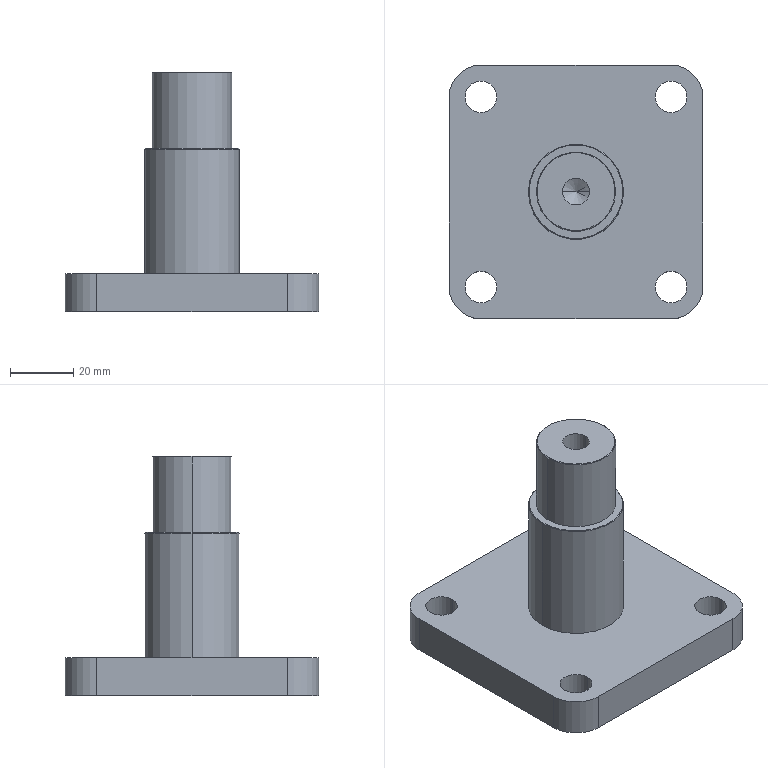Part | NX | features BREP 2 | 2 solids | 38 faces | box 80 x 80 x 75.5 mm | volume 109108 mm3 | cylinder 22 | plane 10 | cone 6 | commonest cylinder face diameters 10 x8 25 x6 20 x4 8.5 x2 30 x2
STEP:
#1=CARTESIAN_POINT('',(-25.,30.,0.));
#2=VERTEX_POINT('',#1);
#3=CARTESIAN_POINT('',(-35.,30.,0.));
#4=VERTEX_POINT('',#3);
#5=CARTESIAN_POINT('',(-30.,30.,0.));
#6=DIRECTION('',(0.,0.,-1.));
#7=DIRECTION('',(-1.,0.,0.));
#8=AXIS2_PLACEMENT_3D('',#5,#6,#7);
#9=CIRCLE('',#8,5.);
#10=EDGE_CURVE('',#2,#4,#9,.T.);
#11=ORIENTED_EDGE('',*,*,#10,.T.);
#12=CARTESIAN_POINT('',(-35.,30.,12.));
#13=VERTEX_POINT('',#12);
#14=CARTESIAN_POINT('',(-35.,30.,12.));
#15=DIRECTION('',(0.,0.,1.));
#16=VECTOR('',#15,1000.);
#17=LINE('',#14,#16);
#18=EDGE_CURVE('',#13,#4,#17,.F.);
#19=ORIENTED_EDGE('',*,*,#18,.F.);
#20=CARTESIAN_POINT('',(-25.,30.,12.));
#21=VERTEX_POINT('',#20);
#22=CARTESIAN_POINT('',(-30.,30.,12.));
#23=DIRECTION('',(0.,0.,1.));
#24=DIRECTION('',(1.,0.,0.));
#25=AXIS2_PLACEMENT_3D('',#22,#23,#24);
#26=CIRCLE('',#25,5.);
#27=EDGE_CURVE('',#13,#21,#26,.T.);
#28=ORIENTED_EDGE('',*,*,#27,.T.);
#29=CARTESIAN_POINT('',(-25.,30.,12.));
#30=DIRECTION('',(0.,0.,1.));
#31=VECTOR('',#30,1000.);
#32=LINE('',#29,#31);
#33=EDGE_CURVE('',#21,#2,#32,.F.);
#34=ORIENTED_EDGE('',*,*,#33,.T.);
#35=EDGE_LOOP('',(#11,#19,#28,#34));
#36=FACE_BOUND('',#35,.T.);
#37=CARTESIAN_POINT('',(-30.,30.,12.));
#38=DIRECTION('',(0.,0.,1.));
#39=DIRECTION('',(1.,0.,0.));
#40=AXIS2_PLACEMENT_3D('',#37,#38,#39);
#41=CYLINDRICAL_SURFACE('',#40,5.);
#42=ADVANCED_FACE('',(#36),#41,.F.);
#43=CARTESIAN_POINT('',(35.,-30.,0.));
#44=VERTEX_POINT('',#43);
#45=CARTESIAN_POINT('',(25.,-30.,0.));
#46=VERTEX_POINT('',#45);
#47=CARTESIAN_POINT('',(30.,-30.,0.));
#48=DIRECTION('',(0.,0.,-1.));
#49=DIRECTION('',(-1.,0.,0.));
#50=AXIS2_PLACEMENT_3D('',#47,#48,#49);
#51=CIRCLE('',#50,5.);
#52=EDGE_CURVE('',#44,#46,#51,.T.);
#53=ORIENTED_EDGE('',*,*,#52,.T.);
#54=CARTESIAN_POINT('',(25.,-30.,12.));
#55=VERTEX_POINT('',#54);
#56=CARTESIAN_POINT('',(25.,-30.,12.));
#57=DIRECTION('',(0.,0.,1.));
#58=VECTOR('',#57,1000.);
#59=LINE('',#56,#58);
#60=EDGE_CURVE('',#55,#46,#59,.F.);
#61=ORIENTED_EDGE('',*,*,#60,.F.);
#62=CARTESIAN_POINT('',(35.,-30.,12.));
#63=VERTEX_POINT('',#62);
#64=CARTESIAN_POINT('',(30.,-30.,12.));
#65=DIRECTION('',(0.,0.,1.));
#66=DIRECTION('',(1.,0.,0.));
#67=AXIS2_PLACEMENT_3D('',#64,#65,#66);
#68=CIRCLE('',#67,5.);
#69=EDGE_CURVE('',#55,#63,#68,.T.);
#70=ORIENTED_EDGE('',*,*,#69,.T.);
#71=CARTESIAN_POINT('',(35.,-30.,12.));
#72=DIRECTION('',(0.,0.,1.));
#73=VECTOR('',#72,1000.);
#74=LINE('',#71,#73);
#75=EDGE_CURVE('',#63,#44,#74,.F.);
#76=ORIENTED_EDGE('',*,*,#75,.T.);
#77=EDGE_LOOP('',(#53,#61,#70,#76));
#78=FACE_BOUND('',#77,.T.);
#79=CARTESIAN_POINT('',(30.,-30.,12.));
#80=DIRECTION('',(0.,0.,1.));
#81=DIRECTION('',(1.,0.,0.));
#82=AXIS2_PLACEMENT_3D('',#79,#80,#81);
#83=CYLINDRICAL_SURFACE('',#82,5.);
#84=ADVANCED_FACE('',(#78),#83,.F.);
#85=CARTESIAN_POINT('',(-25.,-30.,0.));
#86=VERTEX_POINT('',#85);
#87=CARTESIAN_POINT('',(-35.,-30.,0.));
#88=VERTEX_POINT('',#87);
#89=CARTESIAN_POINT('',(-30.,-30.,0.));
#90=DIRECTION('',(0.,0.,-1.));
#91=DIRECTION('',(-1.,0.,0.));
#92=AXIS2_PLACEMENT_3D('',#89,#90,#91);
#93=CIRCLE('',#92,5.);
#94=EDGE_CURVE('',#86,#88,#93,.T.);
#95=ORIENTED_EDGE('',*,*,#94,.T.);
#96=CARTESIAN_POINT('',(-35.,-30.,12.));
#97=VERTEX_POINT('',#96);
#98=CARTESIAN_POINT('',(-35.,-30.,12.));
#99=DIRECTION('',(0.,0.,1.));
#100=VECTOR('',#99,1000.);
#101=LINE('',#98,#100);
#102=EDGE_CURVE('',#97,#88,#101,.F.);
#103=ORIENTED_EDGE('',*,*,#102,.F.);
#104=CARTESIAN_POINT('',(-25.,-30.,12.));
#105=VERTEX_POINT('',#104);
#106=CARTESIAN_POINT('',(-30.,-30.,12.));
#107=DIRECTION('',(0.,0.,1.));
#108=DIRECTION('',(1.,0.,0.));
#109=AXIS2_PLACEMENT_3D('',#106,#107,#108);
#110=CIRCLE('',#109,5.);
#111=EDGE_CURVE('',#97,#105,#110,.T.);
#112=ORIENTED_EDGE('',*,*,#111,.T.);
#113=CARTESIAN_POINT('',(-25.,-30.,12.));
#114=DIRECTION('',(0.,0.,1.));
#115=VECTOR('',#114,1000.);
#116=LINE('',#113,#115);
#117=EDGE_CURVE('',#105,#86,#116,.F.);
#118=ORIENTED_EDGE('',*,*,#117,.T.);
#119=EDGE_LOOP('',(#95,#103,#112,#118));
#120=FACE_BOUND('',#119,.T.);
#121=CARTESIAN_POINT('',(-30.,-30.,12.));
#122=DIRECTION('',(0.,0.,1.));
#123=DIRECTION('',(1.,0.,0.));
#124=AXIS2_PLACEMENT_3D('',#121,#122,#123);
#125=CYLINDRICAL_SURFACE('',#124,5.);
#126=ADVANCED_FACE('',(#120),#125,.F.);
#127=CARTESIAN_POINT('',(35.,30.,0.));
#128=VERTEX_POINT('',#127);
#129=CARTESIAN_POINT('',(25.,30.,0.));
#130=VERTEX_POINT('',#129);
#131=CARTESIAN_POINT('',(30.,30.,0.));
#132=DIRECTION('',(0.,0.,-1.));
#133=DIRECTION('',(-1.,0.,0.));
#134=AXIS2_PLACEMENT_3D('',#131,#132,#133);
#135=CIRCLE('',#134,5.);
#136=EDGE_CURVE('',#128,#130,#135,.T.);
#137=ORIENTED_EDGE('',*,*,#136,.T.);
#138=CARTESIAN_POINT('',(25.,30.,12.));
#139=VERTEX_POINT('',#138);
#140=CARTESIAN_POINT('',(25.,30.,12.));
#141=DIRECTION('',(0.,0.,1.));
#142=VECTOR('',#141,1000.);
#143=LINE('',#140,#142);
#144=EDGE_CURVE('',#139,#130,#143,.F.);
#145=ORIENTED_EDGE('',*,*,#144,.F.);
#146=CARTESIAN_POINT('',(35.,30.,12.));
#147=VERTEX_POINT('',#146);
#148=CARTESIAN_POINT('',(30.,30.,12.));
#149=DIRECTION('',(0.,0.,1.));
#150=DIRECTION('',(1.,0.,0.));
#151=AXIS2_PLACEMENT_3D('',#148,#149,#150);
#152=CIRCLE('',#151,5.);
#153=EDGE_CURVE('',#139,#147,#152,.T.);
#154=ORIENTED_EDGE('',*,*,#153,.T.);
#155=CARTESIAN_POINT('',(35.,30.,12.));
#156=DIRECTION('',(0.,0.,1.));
#157=VECTOR('',#156,1000.);
#158=LINE('',#155,#157);
#159=EDGE_CURVE('',#147,#128,#158,.F.);
#160=ORIENTED_EDGE('',*,*,#159,.T.);
#161=EDGE_LOOP('',(#137,#145,#154,#160));
#162=FACE_BOUND('',#161,.T.);
#163=CARTESIAN_POINT('',(30.,30.,12.));
#164=DIRECTION('',(0.,0.,1.));
#165=DIRECTION('',(1.,0.,0.));
#166=AXIS2_PLACEMENT_3D('',#163,#164,#165);
#167=CYLINDRICAL_SURFACE('',#166,5.);
#168=ADVANCED_FACE('',(#162),#167,.F.);
#169=CARTESIAN_POINT('',(-12.5,0.,0.));
#170=VERTEX_POINT('',#169);
#171=CARTESIAN_POINT('',(12.5,0.,0.));
#172=VERTEX_POINT('',#171);
#173=CARTESIAN_POINT('',(0.,0.,0.));
#174=DIRECTION('',(0.,0.,1.));
#175=DIRECTION('',(1.,0.,0.));
#176=AXIS2_PLACEMENT_3D('',#173,#174,#175);
#177=CIRCLE('',#176,12.5);
#178=EDGE_CURVE('',#170,#172,#177,.T.);
#179=ORIENTED_EDGE('',*,*,#178,.F.);
#180=CARTESIAN_POINT('',(-12.5,0.,12.));
#181=VERTEX_POINT('',#180);
#182=CARTESIAN_POINT('',(-12.5,0.,0.));
#183=DIRECTION('',(0.,0.,1.));
#184=VECTOR('',#183,1000.);
#185=LINE('',#182,#184);
#186=EDGE_CURVE('',#181,#170,#185,.F.);
#187=ORIENTED_EDGE('',*,*,#186,.F.);
#188=CARTESIAN_POINT('',(12.5,0.,12.));
#189=VERTEX_POINT('',#188);
#190=CARTESIAN_POINT('',(0.,0.,12.));
#191=DIRECTION('',(0.,0.,1.));
#192=DIRECTION('',(1.,0.,0.));
#193=AXIS2_PLACEMENT_3D('',#190,#191,#192);
#194=CIRCLE('',#193,12.5);
#195=EDGE_CURVE('',#181,#189,#194,.T.);
#196=ORIENTED_EDGE('',*,*,#195,.T.);
#197=CARTESIAN_POINT('',(12.5,0.,0.));
#198=DIRECTION('',(0.,0.,1.));
#199=VECTOR('',#198,1000.);
#200=LINE('',#197,#199);
#201=EDGE_CURVE('',#189,#172,#200,.F.);
#202=ORIENTED_EDGE('',*,*,#201,.T.);
#203=EDGE_LOOP('',(#179,#187,#196,#202));
#204=FACE_BOUND('',#203,.T.);
#205=CARTESIAN_POINT('',(0.,0.,0.));
#206=DIRECTION('',(0.,0.,1.));
#207=DIRECTION('',(1.,0.,0.));
#208=AXIS2_PLACEMENT_3D('',#205,#206,#207);
#209=CYLINDRICAL_SURFACE('',#208,12.5);
#210=ADVANCED_FACE('',(#204),#209,.F.);
#211=CARTESIAN_POINT('',(-30.,-40.,12.));
#212=VERTEX_POINT('',#211);
#213=CARTESIAN_POINT('',(30.,-40.,12.));
#214=VERTEX_POINT('',#213);
#215=CARTESIAN_POINT('',(-40.,-40.,12.));
#216=DIRECTION('',(1.,0.,0.));
#217=VECTOR('',#216,1000.);
#218=LINE('',#215,#217);
#219=EDGE_CURVE('',#212,#214,#218,.T.);
#220=ORIENTED_EDGE('',*,*,#219,.T.);
#221=CARTESIAN_POINT('',(40.,-30.,12.));
#222=VERTEX_POINT('',#221);
#223=CARTESIAN_POINT('',(30.,-30.,12.));
#224=DIRECTION('',(0.,0.,1.));
#225=DIRECTION('',(-1.,0.,0.));
#226=AXIS2_PLACEMENT_3D('',#223,#224,#225);
#227=CIRCLE('',#226,10.);
#228=EDGE_CURVE('',#214,#222,#227,.T.);
#229=ORIENTED_EDGE('',*,*,#228,.T.);
#230=CARTESIAN_POINT('',(40.,30.,12.));
#231=VERTEX_POINT('',#230);
#232=CARTESIAN_POINT('',(40.,-40.,12.));
#233=DIRECTION('',(0.,1.,0.));
#234=VECTOR('',#233,1000.);
#235=LINE('',#232,#234);
#236=EDGE_CURVE('',#222,#231,#235,.T.);
#237=ORIENTED_EDGE('',*,*,#236,.T.);
#238=CARTESIAN_POINT('',(30.,40.,12.));
#239=VERTEX_POINT('',#238);
#240=CARTESIAN_POINT('',(30.,30.,12.));
#241=DIRECTION('',(0.,0.,1.));
#242=DIRECTION('',(-1.,0.,0.));
#243=AXIS2_PLACEMENT_3D('',#240,#241,#242);
#244=CIRCLE('',#243,10.);
#245=EDGE_CURVE('',#231,#239,#244,.T.);
#246=ORIENTED_EDGE('',*,*,#245,.T.);
#247=CARTESIAN_POINT('',(-30.,40.,12.));
#248=VERTEX_POINT('',#247);
#249=CARTESIAN_POINT('',(-40.,40.,12.));
#250=DIRECTION('',(-1.,0.,0.));
#251=VECTOR('',#250,1000.);
#252=LINE('',#249,#251);
#253=EDGE_CURVE('',#239,#248,#252,.T.);
#254=ORIENTED_EDGE('',*,*,#253,.T.);
#255=CARTESIAN_POINT('',(-40.,30.,12.));
#256=VERTEX_POINT('',#255);
#257=CARTESIAN_POINT('',(-30.,30.,12.));
#258=DIRECTION('',(0.,0.,1.));
#259=DIRECTION('',(-1.,0.,0.));
#260=AXIS2_PLACEMENT_3D('',#257,#258,#259);
#261=CIRCLE('',#260,10.);
#262=EDGE_CURVE('',#248,#256,#261,.T.);
#263=ORIENTED_EDGE('',*,*,#262,.T.);
#264=CARTESIAN_POINT('',(-40.,-30.,12.));
#265=VERTEX_POINT('',#264);
#266=CARTESIAN_POINT('',(-40.,-40.,12.));
#267=DIRECTION('',(0.,-1.,0.));
#268=VECTOR('',#267,1000.);
#269=LINE('',#266,#268);
#270=EDGE_CURVE('',#256,#265,#269,.T.);
#271=ORIENTED_EDGE('',*,*,#270,.T.);
#272=CARTESIAN_POINT('',(-30.,-30.,12.));
#273=DIRECTION('',(0.,0.,1.));
#274=DIRECTION('',(-1.,0.,0.));
#275=AXIS2_PLACEMENT_3D('',#272,#273,#274);
#276=CIRCLE('',#275,10.);
#277=EDGE_CURVE('',#265,#212,#276,.T.);
#278=ORIENTED_EDGE('',*,*,#277,.T.);
#279=EDGE_LOOP('',(#220,#229,#237,#246,#254,#263,#271,#278));
#280=FACE_BOUND('',#279,.T.);
#281=CARTESIAN_POINT('',(-30.,-30.,12.));
#282=DIRECTION('',(0.,0.,1.));
#283=DIRECTION('',(1.,0.,0.));
#284=AXIS2_PLACEMENT_3D('',#281,#282,#283);
#285=CIRCLE('',#284,5.);
#286=EDGE_CURVE('',#105,#97,#285,.T.);
#287=ORIENTED_EDGE('',*,*,#286,.F.);
#288=ORIENTED_EDGE('',*,*,#111,.F.);
#289=EDGE_LOOP('',(#287,#288));
#290=FACE_BOUND('',#289,.T.);
#291=CARTESIAN_POINT('',(30.,30.,12.));
#292=DIRECTION('',(0.,0.,1.));
#293=DIRECTION('',(1.,0.,0.));
#294=AXIS2_PLACEMENT_3D('',#291,#292,#293);
#295=CIRCLE('',#294,5.);
#296=EDGE_CURVE('',#147,#139,#295,.T.);
#297=ORIENTED_EDGE('',*,*,#296,.F.);
#298=ORIENTED_EDGE('',*,*,#153,.F.);
#299=EDGE_LOOP('',(#297,#298));
#300=FACE_BOUND('',#299,.T.);
#301=CARTESIAN_POINT('',(0.,0.,12.));
#302=DIRECTION('',(0.,0.,1.));
#303=DIRECTION('',(1.,0.,0.));
#304=AXIS2_PLACEMENT_3D('',#301,#302,#303);
#305=CIRCLE('',#304,12.5);
#306=EDGE_CURVE('',#189,#181,#305,.T.);
#307=ORIENTED_EDGE('',*,*,#306,.F.);
#308=ORIENTED_EDGE('',*,*,#195,.F.);
#309=EDGE_LOOP('',(#307,#308));
#310=FACE_BOUND('',#309,.T.);
#311=CARTESIAN_POINT('',(30.,-30.,12.));
#312=DIRECTION('',(0.,0.,1.));
#313=DIRECTION('',(1.,0.,0.));
#314=AXIS2_PLACEMENT_3D('',#311,#312,#313);
#315=CIRCLE('',#314,5.);
#316=EDGE_CURVE('',#63,#55,#315,.T.);
#317=ORIENTED_EDGE('',*,*,#316,.F.);
#318=ORIENTED_EDGE('',*,*,#69,.F.);
#319=EDGE_LOOP('',(#317,#318));
#320=FACE_BOUND('',#319,.T.);
#321=CARTESIAN_POINT('',(-30.,30.,12.));
#322=DIRECTION('',(0.,0.,1.));
#323=DIRECTION('',(1.,0.,0.));
#324=AXIS2_PLACEMENT_3D('',#321,#322,#323);
#325=CIRCLE('',#324,5.);
#326=EDGE_CURVE('',#21,#13,#325,.T.);
#327=ORIENTED_EDGE('',*,*,#326,.F.);
#328=ORIENTED_EDGE('',*,*,#27,.F.);
#329=EDGE_LOOP('',(#327,#328));
#330=FACE_BOUND('',#329,.T.);
#331=CARTESIAN_POINT('',(0.,0.,12.));
#332=DIRECTION('',(0.,0.,-1.));
#333=DIRECTION('',(0.,-1.,0.));
#334=AXIS2_PLACEMENT_3D('',#331,#332,#333);
#335=PLANE('',#334);
#336=ADVANCED_FACE('',(#280,#290,#300,#310,#320,#330),#335,.F.);
#337=ORIENTED_EDGE('',*,*,#236,.F.);
#338=CARTESIAN_POINT('',(40.,-30.,0.));
#339=VERTEX_POINT('',#338);
#340=CARTESIAN_POINT('',(40.,-30.,12.));
#341=DIRECTION('',(0.,0.,-1.));
#342=VECTOR('',#341,1000.);
#343=LINE('',#340,#342);
#344=EDGE_CURVE('',#222,#339,#343,.T.);
#345=ORIENTED_EDGE('',*,*,#344,.T.);
#346=CARTESIAN_POINT('',(40.,30.,0.));
#347=VERTEX_POINT('',#346);
#348=CARTESIAN_POINT('',(40.,-40.,0.));
#349=DIRECTION('',(0.,1.,0.));
#350=VECTOR('',#349,1000.);
#351=LINE('',#348,#350);
#352=EDGE_CURVE('',#339,#347,#351,.T.);
#353=ORIENTED_EDGE('',*,*,#352,.T.);
#354=CARTESIAN_POINT('',(40.,30.,12.));
#355=DIRECTION('',(0.,0.,1.));
#356=VECTOR('',#355,1000.);
#357=LINE('',#354,#356);
#358=EDGE_CURVE('',#347,#231,#357,.T.);
#359=ORIENTED_EDGE('',*,*,#358,.T.);
#360=EDGE_LOOP('',(#337,#345,#353,#359));
#361=FACE_BOUND('',#360,.T.);
#362=CARTESIAN_POINT('',(40.,-40.,12.));
#363=DIRECTION('',(-1.,0.,0.));
#364=DIRECTION('',(0.,0.,1.));
#365=AXIS2_PLACEMENT_3D('',#362,#363,#364);
#366=PLANE('',#365);
#367=ADVANCED_FACE('',(#361),#366,.F.);
#368=CARTESIAN_POINT('',(30.,40.,0.));
#369=VERTEX_POINT('',#368);
#370=CARTESIAN_POINT('',(-30.,40.,0.));
#371=VERTEX_POINT('',#370);
#372=CARTESIAN_POINT('',(-40.,40.,0.));
#373=DIRECTION('',(-1.,0.,0.));
#374=VECTOR('',#373,1000.);
#375=LINE('',#372,#374);
#376=EDGE_CURVE('',#369,#371,#375,.T.);
#377=ORIENTED_EDGE('',*,*,#376,.T.);
#378=CARTESIAN_POINT('',(-30.,40.,12.));
#379=DIRECTION('',(0.,0.,1.));
#380=VECTOR('',#379,1000.);
#381=LINE('',#378,#380);
#382=EDGE_CURVE('',#371,#248,#381,.T.);
#383=ORIENTED_EDGE('',*,*,#382,.T.);
#384=ORIENTED_EDGE('',*,*,#253,.F.);
#385=CARTESIAN_POINT('',(30.,40.,12.));
#386=DIRECTION('',(0.,0.,-1.));
#387=VECTOR('',#386,1000.);
#388=LINE('',#385,#387);
#389=EDGE_CURVE('',#239,#369,#388,.T.);
#390=ORIENTED_EDGE('',*,*,#389,.T.);
#391=EDGE_LOOP('',(#377,#383,#384,#390));
#392=FACE_BOUND('',#391,.T.);
#393=CARTESIAN_POINT('',(-40.,40.,12.));
#394=DIRECTION('',(0.,-1.,0.));
#395=DIRECTION('',(0.,0.,-1.));
#396=AXIS2_PLACEMENT_3D('',#393,#394,#395);
#397=PLANE('',#396);
#398=ADVANCED_FACE('',(#392),#397,.F.);
#399=CARTESIAN_POINT('',(-40.,30.,0.));
#400=VERTEX_POINT('',#399);
#401=CARTESIAN_POINT('',(-40.,-30.,0.));
#402=VERTEX_POINT('',#401);
#403=CARTESIAN_POINT('',(-40.,-40.,0.));
#404=DIRECTION('',(0.,-1.,0.));
#405=VECTOR('',#404,1000.);
#406=LINE('',#403,#405);
#407=EDGE_CURVE('',#400,#402,#406,.T.);
#408=ORIENTED_EDGE('',*,*,#407,.T.);
#409=CARTESIAN_POINT('',(-40.,-30.,12.));
#410=DIRECTION('',(0.,0.,1.));
#411=VECTOR('',#410,1000.);
#412=LINE('',#409,#411);
#413=EDGE_CURVE('',#402,#265,#412,.T.);
#414=ORIENTED_EDGE('',*,*,#413,.T.);
#415=ORIENTED_EDGE('',*,*,#270,.F.);
#416=CARTESIAN_POINT('',(-40.,30.,12.));
#417=DIRECTION('',(0.,0.,-1.));
#418=VECTOR('',#417,1000.);
#419=LINE('',#416,#418);
#420=EDGE_CURVE('',#256,#400,#419,.T.);
#421=ORIENTED_EDGE('',*,*,#420,.T.);
#422=EDGE_LOOP('',(#408,#414,#415,#421));
#423=FACE_BOUND('',#422,.T.);
#424=CARTESIAN_POINT('',(-40.,-40.,12.));
#425=DIRECTION('',(1.,0.,0.));
#426=DIRECTION('',(0.,1.,0.));
#427=AXIS2_PLACEMENT_3D('',#424,#425,#426);
#428=PLANE('',#427);
#429=ADVANCED_FACE('',(#423),#428,.F.);
#430=CARTESIAN_POINT('',(-30.,-40.,0.));
#431=VERTEX_POINT('',#430);
#432=CARTESIAN_POINT('',(30.,-40.,0.));
#433=VERTEX_POINT('',#432);
#434=CARTESIAN_POINT('',(-40.,-40.,0.));
#435=DIRECTION('',(1.,0.,0.));
#436=VECTOR('',#435,1000.);
#437=LINE('',#434,#436);
#438=EDGE_CURVE('',#431,#433,#437,.T.);
#439=ORIENTED_EDGE('',*,*,#438,.T.);
#440=CARTESIAN_POINT('',(30.,-40.,12.));
#441=DIRECTION('',(0.,0.,1.));
#442=VECTOR('',#441,1000.);
#443=LINE('',#440,#442);
#444=EDGE_CURVE('',#433,#214,#443,.T.);
#445=ORIENTED_EDGE('',*,*,#444,.T.);
#446=ORIENTED_EDGE('',*,*,#219,.F.);
#447=CARTESIAN_POINT('',(-30.,-40.,12.));
#448=DIRECTION('',(0.,0.,-1.));
#449=VECTOR('',#448,1000.);
#450=LINE('',#447,#449);
#451=EDGE_CURVE('',#212,#431,#450,.T.);
#452=ORIENTED_EDGE('',*,*,#451,.T.);
#453=EDGE_LOOP('',(#439,#445,#446,#452));
#454=FACE_BOUND('',#453,.T.);
#455=CARTESIAN_POINT('',(-40.,-40.,12.));
#456=DIRECTION('',(0.,1.,0.));
#457=DIRECTION('',(1.,0.,0.));
#458=AXIS2_PLACEMENT_3D('',#455,#456,#457);
#459=PLANE('',#458);
#460=ADVANCED_FACE('',(#454),#459,.F.);
#461=ORIENTED_EDGE('',*,*,#352,.F.);
#462=CARTESIAN_POINT('',(30.,-30.,0.));
#463=DIRECTION('',(0.,0.,-1.));
#464=DIRECTION('',(-1.,0.,0.));
#465=AXIS2_PLACEMENT_3D('',#462,#463,#464);
#466=CIRCLE('',#465,10.);
#467=EDGE_CURVE('',#339,#433,#466,.T.);
#468=ORIENTED_EDGE('',*,*,#467,.T.);
#469=ORIENTED_EDGE('',*,*,#438,.F.);
#470=CARTESIAN_POINT('',(-30.,-30.,0.));
#471=DIRECTION('',(0.,0.,-1.));
#472=DIRECTION('',(-1.,0.,0.));
#473=AXIS2_PLACEMENT_3D('',#470,#471,#472);
#474=CIRCLE('',#473,10.);
#475=EDGE_CURVE('',#431,#402,#474,.T.);
#476=ORIENTED_EDGE('',*,*,#475,.T.);
#477=ORIENTED_EDGE('',*,*,#407,.F.);
#478=CARTESIAN_POINT('',(-30.,30.,0.));
#479=DIRECTION('',(0.,0.,-1.));
#480=DIRECTION('',(-1.,0.,0.));
#481=AXIS2_PLACEMENT_3D('',#478,#479,#480);
#482=CIRCLE('',#481,10.);
#483=EDGE_CURVE('',#400,#371,#482,.T.);
#484=ORIENTED_EDGE('',*,*,#483,.T.);
#485=ORIENTED_EDGE('',*,*,#376,.F.);
#486=CARTESIAN_POINT('',(30.,30.,0.));
#487=DIRECTION('',(0.,0.,-1.));
#488=DIRECTION('',(-1.,0.,0.));
#489=AXIS2_PLACEMENT_3D('',#486,#487,#488);
#490=CIRCLE('',#489,10.);
#491=EDGE_CURVE('',#369,#347,#490,.T.);
#492=ORIENTED_EDGE('',*,*,#491,.T.);
#493=EDGE_LOOP('',(#461,#468,#469,#476,#477,#484,#485,#492));
#494=FACE_BOUND('',#493,.T.);
#495=ORIENTED_EDGE('',*,*,#10,.F.);
#496=CARTESIAN_POINT('',(-30.,30.,0.));
#497=DIRECTION('',(0.,0.,-1.));
#498=DIRECTION('',(-1.,0.,0.));
#499=AXIS2_PLACEMENT_3D('',#496,#497,#498);
#500=CIRCLE('',#499,5.);
#501=EDGE_CURVE('',#4,#2,#500,.T.);
#502=ORIENTED_EDGE('',*,*,#501,.F.);
#503=EDGE_LOOP('',(#495,#502));
#504=FACE_BOUND('',#503,.T.);
#505=ORIENTED_EDGE('',*,*,#52,.F.);
#506=CARTESIAN_POINT('',(30.,-30.,0.));
#507=DIRECTION('',(0.,0.,-1.));
#508=DIRECTION('',(-1.,0.,0.));
#509=AXIS2_PLACEMENT_3D('',#506,#507,#508);
#510=CIRCLE('',#509,5.);
#511=EDGE_CURVE('',#46,#44,#510,.T.);
#512=ORIENTED_EDGE('',*,*,#511,.F.);
#513=EDGE_LOOP('',(#505,#512));
#514=FACE_BOUND('',#513,.T.);
#515=ORIENTED_EDGE('',*,*,#94,.F.);
#516=CARTESIAN_POINT('',(-30.,-30.,0.));
#517=DIRECTION('',(0.,0.,-1.));
#518=DIRECTION('',(-1.,0.,0.));
#519=AXIS2_PLACEMENT_3D('',#516,#517,#518);
#520=CIRCLE('',#519,5.);
#521=EDGE_CURVE('',#88,#86,#520,.T.);
#522=ORIENTED_EDGE('',*,*,#521,.F.);
#523=EDGE_LOOP('',(#515,#522));
#524=FACE_BOUND('',#523,.T.);
#525=ORIENTED_EDGE('',*,*,#136,.F.);
#526=CARTESIAN_POINT('',(30.,30.,0.));
#527=DIRECTION('',(0.,0.,-1.));
#528=DIRECTION('',(-1.,0.,0.));
#529=AXIS2_PLACEMENT_3D('',#526,#527,#528);
#530=CIRCLE('',#529,5.);
#531=EDGE_CURVE('',#130,#128,#530,.T.);
#532=ORIENTED_EDGE('',*,*,#531,.F.);
#533=EDGE_LOOP('',(#525,#532));
#534=FACE_BOUND('',#533,.T.);
#535=CARTESIAN_POINT('',(0.,0.,0.));
#536=DIRECTION('',(0.,0.,1.));
#537=DIRECTION('',(1.,0.,0.));
#538=AXIS2_PLACEMENT_3D('',#535,#536,#537);
#539=CIRCLE('',#538,12.5);
#540=EDGE_CURVE('',#172,#170,#539,.T.);
#541=ORIENTED_EDGE('',*,*,#540,.T.);
#542=ORIENTED_EDGE('',*,*,#178,.T.);
#543=EDGE_LOOP('',(#541,#542));
#544=FACE_BOUND('',#543,.T.);
#545=CARTESIAN_POINT('',(0.,0.,0.));
#546=DIRECTION('',(0.,0.,-1.));
#547=DIRECTION('',(0.,-1.,0.));
#548=AXIS2_PLACEMENT_3D('',#545,#546,#547);
#549=PLANE('',#548);
#550=ADVANCED_FACE('',(#494,#504,#514,#524,#534,#544),#549,.T.);
#551=ORIENTED_EDGE('',*,*,#186,.T.);
#552=ORIENTED_EDGE('',*,*,#540,.F.);
#553=ORIENTED_EDGE('',*,*,#201,.F.);
#554=ORIENTED_EDGE('',*,*,#306,.T.);
#555=EDGE_LOOP('',(#551,#552,#553,#554));
#556=FACE_BOUND('',#555,.T.);
#557=CARTESIAN_POINT('',(0.,0.,0.));
#558=DIRECTION('',(0.,0.,1.));
#559=DIRECTION('',(1.,0.,0.));
#560=AXIS2_PLACEMENT_3D('',#557,#558,#559);
#561=CYLINDRICAL_SURFACE('',#560,12.5);
#562=ADVANCED_FACE('',(#556),#561,.F.);
#563=ORIENTED_EDGE('',*,*,#228,.F.);
#564=ORIENTED_EDGE('',*,*,#444,.F.);
#565=ORIENTED_EDGE('',*,*,#467,.F.);
#566=ORIENTED_EDGE('',*,*,#344,.F.);
#567=EDGE_LOOP('',(#563,#564,#565,#566));
#568=FACE_BOUND('',#567,.T.);
#569=CARTESIAN_POINT('',(30.,-30.,12.));
#570=DIRECTION('',(0.,0.,-1.));
#571=DIRECTION('',(-1.,0.,0.));
#572=AXIS2_PLACEMENT_3D('',#569,#570,#571);
#573=CYLINDRICAL_SURFACE('',#572,10.);
#574=ADVANCED_FACE('',(#568),#573,.T.);
#575=ORIENTED_EDGE('',*,*,#277,.F.);
#576=ORIENTED_EDGE('',*,*,#413,.F.);
#577=ORIENTED_EDGE('',*,*,#475,.F.);
#578=ORIENTED_EDGE('',*,*,#451,.F.);
#579=EDGE_LOOP('',(#575,#576,#577,#578));
#580=FACE_BOUND('',#579,.T.);
#581=CARTESIAN_POINT('',(-30.,-30.,12.));
#582=DIRECTION('',(0.,0.,-1.));
#583=DIRECTION('',(-1.,0.,0.));
#584=AXIS2_PLACEMENT_3D('',#581,#582,#583);
#585=CYLINDRICAL_SURFACE('',#584,10.);
#586=ADVANCED_FACE('',(#580),#585,.T.);
#587=ORIENTED_EDGE('',*,*,#262,.F.);
#588=ORIENTED_EDGE('',*,*,#382,.F.);
#589=ORIENTED_EDGE('',*,*,#483,.F.);
#590=ORIENTED_EDGE('',*,*,#420,.F.);
#591=EDGE_LOOP('',(#587,#588,#589,#590));
#592=FACE_BOUND('',#591,.T.);
#593=CARTESIAN_POINT('',(-30.,30.,12.));
#594=DIRECTION('',(0.,0.,-1.));
#595=DIRECTION('',(-1.,0.,0.));
#596=AXIS2_PLACEMENT_3D('',#593,#594,#595);
#597=CYLINDRICAL_SURFACE('',#596,10.);
#598=ADVANCED_FACE('',(#592),#597,.T.);
#599=ORIENTED_EDGE('',*,*,#245,.F.);
#600=ORIENTED_EDGE('',*,*,#358,.F.);
#601=ORIENTED_EDGE('',*,*,#491,.F.);
#602=ORIENTED_EDGE('',*,*,#389,.F.);
#603=EDGE_LOOP('',(#599,#600,#601,#602));
#604=FACE_BOUND('',#603,.T.);
#605=CARTESIAN_POINT('',(30.,30.,12.));
#606=DIRECTION('',(0.,0.,-1.));
#607=DIRECTION('',(-1.,0.,0.));
#608=AXIS2_PLACEMENT_3D('',#605,#606,#607);
#609=CYLINDRICAL_SURFACE('',#608,10.);
#610=ADVANCED_FACE('',(#604),#609,.T.);
#611=ORIENTED_EDGE('',*,*,#144,.T.);
#612=ORIENTED_EDGE('',*,*,#531,.T.);
#613=ORIENTED_EDGE('',*,*,#159,.F.);
#614=ORIENTED_EDGE('',*,*,#296,.T.);
#615=EDGE_LOOP('',(#611,#612,#613,#614));
#616=FACE_BOUND('',#615,.T.);
#617=CARTESIAN_POINT('',(30.,30.,12.));
#618=DIRECTION('',(0.,0.,1.));
#619=DIRECTION('',(1.,0.,0.));
#620=AXIS2_PLACEMENT_3D('',#617,#618,#619);
#621=CYLINDRICAL_SURFACE('',#620,5.);
#622=ADVANCED_FACE('',(#616),#621,.F.);
#623=ORIENTED_EDGE('',*,*,#102,.T.);
#624=ORIENTED_EDGE('',*,*,#521,.T.);
#625=ORIENTED_EDGE('',*,*,#117,.F.);
#626=ORIENTED_EDGE('',*,*,#286,.T.);
#627=EDGE_LOOP('',(#623,#624,#625,#626));
#628=FACE_BOUND('',#627,.T.);
#629=CARTESIAN_POINT('',(-30.,-30.,12.));
#630=DIRECTION('',(0.,0.,1.));
#631=DIRECTION('',(1.,0.,0.));
#632=AXIS2_PLACEMENT_3D('',#629,#630,#631);
#633=CYLINDRICAL_SURFACE('',#632,5.);
#634=ADVANCED_FACE('',(#628),#633,.F.);
#635=ORIENTED_EDGE('',*,*,#60,.T.);
#636=ORIENTED_EDGE('',*,*,#511,.T.);
#637=ORIENTED_EDGE('',*,*,#75,.F.);
#638=ORIENTED_EDGE('',*,*,#316,.T.);
#639=EDGE_LOOP('',(#635,#636,#637,#638));
#640=FACE_BOUND('',#639,.T.);
#641=CARTESIAN_POINT('',(30.,-30.,12.));
#642=DIRECTION('',(0.,0.,1.));
#643=DIRECTION('',(1.,0.,0.));
#644=AXIS2_PLACEMENT_3D('',#641,#642,#643);
#645=CYLINDRICAL_SURFACE('',#644,5.);
#646=ADVANCED_FACE('',(#640),#645,.F.);
#647=ORIENTED_EDGE('',*,*,#18,.T.);
#648=ORIENTED_EDGE('',*,*,#501,.T.);
#649=ORIENTED_EDGE('',*,*,#33,.F.);
#650=ORIENTED_EDGE('',*,*,#326,.T.);
#651=EDGE_LOOP('',(#647,#648,#649,#650));
#652=FACE_BOUND('',#651,.T.);
#653=CARTESIAN_POINT('',(-30.,30.,12.));
#654=DIRECTION('',(0.,0.,1.));
#655=DIRECTION('',(1.,0.,0.));
#656=AXIS2_PLACEMENT_3D('',#653,#654,#655);
#657=CYLINDRICAL_SURFACE('',#656,5.);
#658=ADVANCED_FACE('',(#652),#657,.F.);
#659=CLOSED_SHELL('',(#42,#84,#126,#168,#210,#336,#367,#398,#429,#460,#550,#562,#574,#586,#598,#610,#622,#634,#646,#658));
#660=MANIFOLD_SOLID_BREP('',#659);
#661=CARTESIAN_POINT('',(12.3,0.,75.5));
#662=VERTEX_POINT('',#661);
#663=CARTESIAN_POINT('',(-12.3,0.,75.5));
#664=VERTEX_POINT('',#663);
#665=CARTESIAN_POINT('',(0.,0.,75.5));
#666=DIRECTION('',(0.,0.,1.));
#667=DIRECTION('',(1.,0.,0.));
#668=AXIS2_PLACEMENT_3D('',#665,#666,#667);
#669=CIRCLE('',#668,12.3);
#670=EDGE_CURVE('',#662,#664,#669,.T.);
#671=ORIENTED_EDGE('',*,*,#670,.F.);
#672=CARTESIAN_POINT('',(12.5,0.,75.3));
#673=VERTEX_POINT('',#672);
#674=CARTESIAN_POINT('',(12.3,0.,75.5));
#675=DIRECTION('',(0.7071,0.,-0.7071));
#676=VECTOR('',#675,1000.);
#677=LINE('',#674,#676);
#678=EDGE_CURVE('',#662,#673,#677,.T.);
#679=ORIENTED_EDGE('',*,*,#678,.T.);
#680=CARTESIAN_POINT('',(-12.5,0.,75.3));
#681=VERTEX_POINT('',#680);
#682=CARTESIAN_POINT('',(0.,0.,75.3));
#683=DIRECTION('',(0.,0.,-1.));
#684=DIRECTION('',(1.,0.,0.));
#685=AXIS2_PLACEMENT_3D('',#682,#683,#684);
#686=CIRCLE('',#685,12.5);
#687=EDGE_CURVE('',#681,#673,#686,.T.);
#688=ORIENTED_EDGE('',*,*,#687,.F.);
#689=CARTESIAN_POINT('',(-12.3,0.,75.5));
#690=DIRECTION('',(-0.7071,0.,-0.7071));
#691=VECTOR('',#690,1000.);
#692=LINE('',#689,#691);
#693=EDGE_CURVE('',#664,#681,#692,.T.);
#694=ORIENTED_EDGE('',*,*,#693,.F.);
#695=EDGE_LOOP('',(#671,#679,#688,#694));
#696=FACE_BOUND('',#695,.T.);
#697=CARTESIAN_POINT('',(0.,0.,75.5));
#698=DIRECTION('',(0.,0.,-1.));
#699=DIRECTION('',(-1.,0.,0.));
#700=AXIS2_PLACEMENT_3D('',#697,#698,#699);
#701=CONICAL_SURFACE('',#700,12.3,0.7854);
#702=ADVANCED_FACE('',(#696),#701,.T.);
#703=CARTESIAN_POINT('',(14.8,0.,51.5));
#704=VERTEX_POINT('',#703);
#705=CARTESIAN_POINT('',(-14.8,0.,51.5));
#706=VERTEX_POINT('',#705);
#707=CARTESIAN_POINT('',(0.,0.,51.5));
#708=DIRECTION('',(0.,0.,1.));
#709=DIRECTION('',(1.,0.,0.));
#710=AXIS2_PLACEMENT_3D('',#707,#708,#709);
#711=CIRCLE('',#710,14.8);
#712=EDGE_CURVE('',#704,#706,#711,.T.);
#713=ORIENTED_EDGE('',*,*,#712,.F.);
#714=CARTESIAN_POINT('',(15.,0.,51.3));
#715=VERTEX_POINT('',#714);
#716=CARTESIAN_POINT('',(14.8,0.,51.5));
#717=DIRECTION('',(0.7071,0.,-0.7071));
#718=VECTOR('',#717,1000.);
#719=LINE('',#716,#718);
#720=EDGE_CURVE('',#704,#715,#719,.T.);
#721=ORIENTED_EDGE('',*,*,#720,.T.);
#722=CARTESIAN_POINT('',(-15.,0.,51.3));
#723=VERTEX_POINT('',#722);
#724=CARTESIAN_POINT('',(0.,0.,51.3));
#725=DIRECTION('',(0.,0.,-1.));
#726=DIRECTION('',(1.,0.,0.));
#727=AXIS2_PLACEMENT_3D('',#724,#725,#726);
#728=CIRCLE('',#727,15.);
#729=EDGE_CURVE('',#723,#715,#728,.T.);
#730=ORIENTED_EDGE('',*,*,#729,.F.);
#731=CARTESIAN_POINT('',(-14.8,0.,51.5));
#732=DIRECTION('',(-0.7071,0.,-0.7071));
#733=VECTOR('',#732,1000.);
#734=LINE('',#731,#733);
#735=EDGE_CURVE('',#706,#723,#734,.T.);
#736=ORIENTED_EDGE('',*,*,#735,.F.);
#737=EDGE_LOOP('',(#713,#721,#730,#736));
#738=FACE_BOUND('',#737,.T.);
#739=CARTESIAN_POINT('',(0.,0.,51.5));
#740=DIRECTION('',(0.,0.,-1.));
#741=DIRECTION('',(-1.,0.,0.));
#742=AXIS2_PLACEMENT_3D('',#739,#740,#741);
#743=CONICAL_SURFACE('',#742,14.8,0.7854);
#744=ADVANCED_FACE('',(#738),#743,.T.);
#745=CARTESIAN_POINT('',(-4.25,0.,48.));
#746=VERTEX_POINT('',#745);
#747=CARTESIAN_POINT('',(4.25,0.,48.));
#748=VERTEX_POINT('',#747);
#749=CARTESIAN_POINT('',(0.,0.,48.));
#750=DIRECTION('',(0.,0.,1.));
#751=DIRECTION('',(1.,0.,0.));
#752=AXIS2_PLACEMENT_3D('',#749,#750,#751);
#753=CIRCLE('',#752,4.25);
#754=EDGE_CURVE('',#746,#748,#753,.T.);
#755=ORIENTED_EDGE('',*,*,#754,.F.);
#756=CARTESIAN_POINT('',(-4.25,0.,75.5));
#757=VERTEX_POINT('',#756);
#758=CARTESIAN_POINT('',(-4.25,0.,75.5));
#759=DIRECTION('',(0.,0.,1.));
#760=VECTOR('',#759,1000.);
#761=LINE('',#758,#760);
#762=EDGE_CURVE('',#757,#746,#761,.F.);
#763=ORIENTED_EDGE('',*,*,#762,.F.);
#764=CARTESIAN_POINT('',(4.25,0.,75.5));
#765=VERTEX_POINT('',#764);
#766=CARTESIAN_POINT('',(0.,0.,75.5));
#767=DIRECTION('',(0.,0.,1.));
#768=DIRECTION('',(1.,0.,0.));
#769=AXIS2_PLACEMENT_3D('',#766,#767,#768);
#770=CIRCLE('',#769,4.25);
#771=EDGE_CURVE('',#757,#765,#770,.T.);
#772=ORIENTED_EDGE('',*,*,#771,.T.);
#773=CARTESIAN_POINT('',(4.25,0.,75.5));
#774=DIRECTION('',(0.,0.,1.));
#775=VECTOR('',#774,1000.);
#776=LINE('',#773,#775);
#777=EDGE_CURVE('',#765,#748,#776,.F.);
#778=ORIENTED_EDGE('',*,*,#777,.T.);
#779=EDGE_LOOP('',(#755,#763,#772,#778));
#780=FACE_BOUND('',#779,.T.);
#781=CARTESIAN_POINT('',(0.,0.,75.5));
#782=DIRECTION('',(0.,0.,1.));
#783=DIRECTION('',(1.,0.,0.));
#784=AXIS2_PLACEMENT_3D('',#781,#782,#783);
#785=CYLINDRICAL_SURFACE('',#784,4.25);
#786=ADVANCED_FACE('',(#780),#785,.F.);
#787=CARTESIAN_POINT('',(0.,0.,45.446));
#788=VERTEX_POINT('',#787);
#789=CARTESIAN_POINT('',(4.25,0.,48.));
#790=DIRECTION('',(0.8572,0.,0.515));
#791=VECTOR('',#790,1000.);
#792=LINE('',#789,#791);
#793=EDGE_CURVE('',#748,#788,#792,.F.);
#794=ORIENTED_EDGE('',*,*,#793,.T.);
#795=CARTESIAN_POINT('',(-4.25,0.,48.));
#796=DIRECTION('',(-0.8572,0.,0.515));
#797=VECTOR('',#796,1000.);
#798=LINE('',#795,#797);
#799=EDGE_CURVE('',#746,#788,#798,.F.);
#800=ORIENTED_EDGE('',*,*,#799,.F.);
#801=ORIENTED_EDGE('',*,*,#754,.T.);
#802=EDGE_LOOP('',(#794,#800,#801));
#803=FACE_BOUND('',#802,.T.);
#804=CARTESIAN_POINT('',(0.,0.,48.));
#805=DIRECTION('',(0.,0.,1.));
#806=DIRECTION('',(1.,0.,0.));
#807=AXIS2_PLACEMENT_3D('',#804,#805,#806);
#808=CONICAL_SURFACE('',#807,4.25,1.03);
#809=ADVANCED_FACE('',(#803),#808,.F.);
#810=ORIENTED_EDGE('',*,*,#687,.T.);
#811=CARTESIAN_POINT('',(12.5,0.,51.5));
#812=VERTEX_POINT('',#811);
#813=CARTESIAN_POINT('',(12.5,0.,75.5));
#814=DIRECTION('',(0.,0.,-1.));
#815=VECTOR('',#814,1000.);
#816=LINE('',#813,#815);
#817=EDGE_CURVE('',#673,#812,#816,.T.);
#818=ORIENTED_EDGE('',*,*,#817,.T.);
#819=CARTESIAN_POINT('',(-12.5,0.,51.5));
#820=VERTEX_POINT('',#819);
#821=CARTESIAN_POINT('',(0.,0.,51.5));
#822=DIRECTION('',(0.,0.,1.));
#823=DIRECTION('',(1.,0.,0.));
#824=AXIS2_PLACEMENT_3D('',#821,#822,#823);
#825=CIRCLE('',#824,12.5);
#826=EDGE_CURVE('',#812,#820,#825,.T.);
#827=ORIENTED_EDGE('',*,*,#826,.T.);
#828=CARTESIAN_POINT('',(-12.5,0.,75.5));
#829=DIRECTION('',(0.,0.,-1.));
#830=VECTOR('',#829,1000.);
#831=LINE('',#828,#830);
#832=EDGE_CURVE('',#681,#820,#831,.T.);
#833=ORIENTED_EDGE('',*,*,#832,.F.);
#834=EDGE_LOOP('',(#810,#818,#827,#833));
#835=FACE_BOUND('',#834,.T.);
#836=CARTESIAN_POINT('',(0.,0.,75.5));
#837=DIRECTION('',(0.,0.,-1.));
#838=DIRECTION('',(-1.,0.,0.));
#839=AXIS2_PLACEMENT_3D('',#836,#837,#838);
#840=CYLINDRICAL_SURFACE('',#839,12.5);
#841=ADVANCED_FACE('',(#835),#840,.T.);
#842=ORIENTED_EDGE('',*,*,#729,.T.);
#843=CARTESIAN_POINT('',(15.,0.,12.));
#844=VERTEX_POINT('',#843);
#845=CARTESIAN_POINT('',(15.,0.,51.5));
#846=DIRECTION('',(0.,0.,-1.));
#847=VECTOR('',#846,1000.);
#848=LINE('',#845,#847);
#849=EDGE_CURVE('',#715,#844,#848,.T.);
#850=ORIENTED_EDGE('',*,*,#849,.T.);
#851=CARTESIAN_POINT('',(-15.,0.,12.));
#852=VERTEX_POINT('',#851);
#853=CARTESIAN_POINT('',(0.,0.,12.));
#854=DIRECTION('',(0.,0.,1.));
#855=DIRECTION('',(1.,0.,0.));
#856=AXIS2_PLACEMENT_3D('',#853,#854,#855);
#857=CIRCLE('',#856,15.);
#858=EDGE_CURVE('',#844,#852,#857,.T.);
#859=ORIENTED_EDGE('',*,*,#858,.T.);
#860=CARTESIAN_POINT('',(-15.,0.,51.5));
#861=DIRECTION('',(0.,0.,-1.));
#862=VECTOR('',#861,1000.);
#863=LINE('',#860,#862);
#864=EDGE_CURVE('',#723,#852,#863,.T.);
#865=ORIENTED_EDGE('',*,*,#864,.F.);
#866=EDGE_LOOP('',(#842,#850,#859,#865));
#867=FACE_BOUND('',#866,.T.);
#868=CARTESIAN_POINT('',(0.,0.,51.5));
#869=DIRECTION('',(0.,0.,-1.));
#870=DIRECTION('',(-1.,0.,0.));
#871=AXIS2_PLACEMENT_3D('',#868,#869,#870);
#872=CYLINDRICAL_SURFACE('',#871,15.);
#873=ADVANCED_FACE('',(#867),#872,.T.);
#874=CARTESIAN_POINT('',(12.5,0.,2.));
#875=VERTEX_POINT('',#874);
#876=CARTESIAN_POINT('',(-12.5,0.,2.));
#877=VERTEX_POINT('',#876);
#878=CARTESIAN_POINT('',(0.,0.,2.));
#879=DIRECTION('',(0.,0.,1.));
#880=DIRECTION('',(1.,0.,0.));
#881=AXIS2_PLACEMENT_3D('',#878,#879,#880);
#882=CIRCLE('',#881,12.5);
#883=EDGE_CURVE('',#875,#877,#882,.T.);
#884=ORIENTED_EDGE('',*,*,#883,.T.);
#885=CARTESIAN_POINT('',(-12.5,0.,12.));
#886=VERTEX_POINT('',#885);
#887=CARTESIAN_POINT('',(-12.5,0.,2.));
#888=DIRECTION('',(0.,0.,1.));
#889=VECTOR('',#888,1000.);
#890=LINE('',#887,#889);
#891=EDGE_CURVE('',#886,#877,#890,.F.);
#892=ORIENTED_EDGE('',*,*,#891,.F.);
#893=CARTESIAN_POINT('',(12.5,0.,12.));
#894=VERTEX_POINT('',#893);
#895=CARTESIAN_POINT('',(0.,0.,12.));
#896=DIRECTION('',(0.,0.,1.));
#897=DIRECTION('',(1.,0.,0.));
#898=AXIS2_PLACEMENT_3D('',#895,#896,#897);
#899=CIRCLE('',#898,12.5);
#900=EDGE_CURVE('',#894,#886,#899,.T.);
#901=ORIENTED_EDGE('',*,*,#900,.F.);
#902=CARTESIAN_POINT('',(12.5,0.,2.));
#903=DIRECTION('',(0.,0.,1.));
#904=VECTOR('',#903,1000.);
#905=LINE('',#902,#904);
#906=EDGE_CURVE('',#894,#875,#905,.F.);
#907=ORIENTED_EDGE('',*,*,#906,.T.);
#908=EDGE_LOOP('',(#884,#892,#901,#907));
#909=FACE_BOUND('',#908,.T.);
#910=CARTESIAN_POINT('',(0.,0.,2.));
#911=DIRECTION('',(0.,0.,1.));
#912=DIRECTION('',(1.,0.,0.));
#913=AXIS2_PLACEMENT_3D('',#910,#911,#912);
#914=CYLINDRICAL_SURFACE('',#913,12.5);
#915=ADVANCED_FACE('',(#909),#914,.T.);
#916=ORIENTED_EDGE('',*,*,#891,.T.);
#917=CARTESIAN_POINT('',(0.,0.,2.));
#918=DIRECTION('',(0.,0.,1.));
#919=DIRECTION('',(1.,0.,0.));
#920=AXIS2_PLACEMENT_3D('',#917,#918,#919);
#921=CIRCLE('',#920,12.5);
#922=EDGE_CURVE('',#877,#875,#921,.T.);
#923=ORIENTED_EDGE('',*,*,#922,.T.);
#924=ORIENTED_EDGE('',*,*,#906,.F.);
#925=CARTESIAN_POINT('',(0.,0.,12.));
#926=DIRECTION('',(0.,0.,1.));
#927=DIRECTION('',(1.,0.,0.));
#928=AXIS2_PLACEMENT_3D('',#925,#926,#927);
#929=CIRCLE('',#928,12.5);
#930=EDGE_CURVE('',#886,#894,#929,.T.);
#931=ORIENTED_EDGE('',*,*,#930,.F.);
#932=EDGE_LOOP('',(#916,#923,#924,#931));
#933=FACE_BOUND('',#932,.T.);
#934=CARTESIAN_POINT('',(0.,0.,2.));
#935=DIRECTION('',(0.,0.,1.));
#936=DIRECTION('',(1.,0.,0.));
#937=AXIS2_PLACEMENT_3D('',#934,#935,#936);
#938=CYLINDRICAL_SURFACE('',#937,12.5);
#939=ADVANCED_FACE('',(#933),#938,.T.);
#940=ORIENTED_EDGE('',*,*,#883,.F.);
#941=ORIENTED_EDGE('',*,*,#922,.F.);
#942=EDGE_LOOP('',(#940,#941));
#943=FACE_BOUND('',#942,.T.);
#944=CARTESIAN_POINT('',(0.,0.,2.));
#945=DIRECTION('',(0.,0.,1.));
#946=DIRECTION('',(1.,0.,0.));
#947=AXIS2_PLACEMENT_3D('',#944,#945,#946);
#948=PLANE('',#947);
#949=ADVANCED_FACE('',(#943),#948,.F.);
#950=ORIENTED_EDGE('',*,*,#849,.F.);
#951=CARTESIAN_POINT('',(0.,0.,51.3));
#952=DIRECTION('',(0.,0.,-1.));
#953=DIRECTION('',(1.,0.,0.));
#954=AXIS2_PLACEMENT_3D('',#951,#952,#953);
#955=CIRCLE('',#954,15.);
#956=EDGE_CURVE('',#715,#723,#955,.T.);
#957=ORIENTED_EDGE('',*,*,#956,.T.);
#958=ORIENTED_EDGE('',*,*,#864,.T.);
#959=CARTESIAN_POINT('',(0.,0.,12.));
#960=DIRECTION('',(0.,0.,1.));
#961=DIRECTION('',(1.,0.,0.));
#962=AXIS2_PLACEMENT_3D('',#959,#960,#961);
#963=CIRCLE('',#962,15.);
#964=EDGE_CURVE('',#852,#844,#963,.T.);
#965=ORIENTED_EDGE('',*,*,#964,.T.);
#966=EDGE_LOOP('',(#950,#957,#958,#965));
#967=FACE_BOUND('',#966,.T.);
#968=CARTESIAN_POINT('',(0.,0.,51.5));
#969=DIRECTION('',(0.,0.,-1.));
#970=DIRECTION('',(-1.,0.,0.));
#971=AXIS2_PLACEMENT_3D('',#968,#969,#970);
#972=CYLINDRICAL_SURFACE('',#971,15.);
#973=ADVANCED_FACE('',(#967),#972,.T.);
#974=CARTESIAN_POINT('',(0.,0.,51.5));
#975=DIRECTION('',(0.,0.,1.));
#976=DIRECTION('',(1.,0.,0.));
#977=AXIS2_PLACEMENT_3D('',#974,#975,#976);
#978=CIRCLE('',#977,14.8);
#979=EDGE_CURVE('',#706,#704,#978,.T.);
#980=ORIENTED_EDGE('',*,*,#979,.T.);
#981=ORIENTED_EDGE('',*,*,#712,.T.);
#982=EDGE_LOOP('',(#980,#981));
#983=FACE_BOUND('',#982,.T.);
#984=CARTESIAN_POINT('',(0.,0.,51.5));
#985=DIRECTION('',(0.,0.,1.));
#986=DIRECTION('',(1.,0.,0.));
#987=AXIS2_PLACEMENT_3D('',#984,#985,#986);
#988=CIRCLE('',#987,12.5);
#989=EDGE_CURVE('',#820,#812,#988,.T.);
#990=ORIENTED_EDGE('',*,*,#989,.F.);
#991=ORIENTED_EDGE('',*,*,#826,.F.);
#992=EDGE_LOOP('',(#990,#991));
#993=FACE_BOUND('',#992,.T.);
#994=CARTESIAN_POINT('',(0.,0.,51.5));
#995=DIRECTION('',(0.,0.,1.));
#996=DIRECTION('',(1.,0.,0.));
#997=AXIS2_PLACEMENT_3D('',#994,#995,#996);
#998=PLANE('',#997);
#999=ADVANCED_FACE('',(#983,#993),#998,.T.);
#1000=ORIENTED_EDGE('',*,*,#964,.F.);
#1001=ORIENTED_EDGE('',*,*,#858,.F.);
#1002=EDGE_LOOP('',(#1000,#1001));
#1003=FACE_BOUND('',#1002,.T.);
#1004=ORIENTED_EDGE('',*,*,#900,.T.);
#1005=ORIENTED_EDGE('',*,*,#930,.T.);
#1006=EDGE_LOOP('',(#1004,#1005));
#1007=FACE_BOUND('',#1006,.T.);
#1008=CARTESIAN_POINT('',(0.,0.,12.));
#1009=DIRECTION('',(0.,0.,1.));
#1010=DIRECTION('',(1.,0.,0.));
#1011=AXIS2_PLACEMENT_3D('',#1008,#1009,#1010);
#1012=PLANE('',#1011);
#1013=ADVANCED_FACE('',(#1003,#1007),#1012,.F.);
#1014=ORIENTED_EDGE('',*,*,#817,.F.);
#1015=CARTESIAN_POINT('',(0.,0.,75.3));
#1016=DIRECTION('',(0.,0.,-1.));
#1017=DIRECTION('',(1.,0.,0.));
#1018=AXIS2_PLACEMENT_3D('',#1015,#1016,#1017);
#1019=CIRCLE('',#1018,12.5);
#1020=EDGE_CURVE('',#673,#681,#1019,.T.);
#1021=ORIENTED_EDGE('',*,*,#1020,.T.);
#1022=ORIENTED_EDGE('',*,*,#832,.T.);
#1023=ORIENTED_EDGE('',*,*,#989,.T.);
#1024=EDGE_LOOP('',(#1014,#1021,#1022,#1023));
#1025=FACE_BOUND('',#1024,.T.);
#1026=CARTESIAN_POINT('',(0.,0.,75.5));
#1027=DIRECTION('',(0.,0.,-1.));
#1028=DIRECTION('',(-1.,0.,0.));
#1029=AXIS2_PLACEMENT_3D('',#1026,#1027,#1028);
#1030=CYLINDRICAL_SURFACE('',#1029,12.5);
#1031=ADVANCED_FACE('',(#1025),#1030,.T.);
#1032=CARTESIAN_POINT('',(0.,0.,75.5));
#1033=DIRECTION('',(0.,0.,1.));
#1034=DIRECTION('',(1.,0.,0.));
#1035=AXIS2_PLACEMENT_3D('',#1032,#1033,#1034);
#1036=CIRCLE('',#1035,12.3);
#1037=EDGE_CURVE('',#664,#662,#1036,.T.);
#1038=ORIENTED_EDGE('',*,*,#1037,.T.);
#1039=ORIENTED_EDGE('',*,*,#670,.T.);
#1040=EDGE_LOOP('',(#1038,#1039));
#1041=FACE_BOUND('',#1040,.T.);
#1042=CARTESIAN_POINT('',(0.,0.,75.5));
#1043=DIRECTION('',(0.,0.,1.));
#1044=DIRECTION('',(1.,0.,0.));
#1045=AXIS2_PLACEMENT_3D('',#1042,#1043,#1044);
#1046=CIRCLE('',#1045,4.25);
#1047=EDGE_CURVE('',#765,#757,#1046,.T.);
#1048=ORIENTED_EDGE('',*,*,#1047,.F.);
#1049=ORIENTED_EDGE('',*,*,#771,.F.);
#1050=EDGE_LOOP('',(#1048,#1049));
#1051=FACE_BOUND('',#1050,.T.);
#1052=CARTESIAN_POINT('',(0.,0.,75.5));
#1053=DIRECTION('',(0.,0.,1.));
#1054=DIRECTION('',(1.,0.,0.));
#1055=AXIS2_PLACEMENT_3D('',#1052,#1053,#1054);
#1056=PLANE('',#1055);
#1057=ADVANCED_FACE('',(#1041,#1051),#1056,.T.);
#1058=ORIENTED_EDGE('',*,*,#799,.T.);
#1059=ORIENTED_EDGE('',*,*,#793,.F.);
#1060=CARTESIAN_POINT('',(0.,0.,48.));
#1061=DIRECTION('',(0.,0.,1.));
#1062=DIRECTION('',(1.,0.,0.));
#1063=AXIS2_PLACEMENT_3D('',#1060,#1061,#1062);
#1064=CIRCLE('',#1063,4.25);
#1065=EDGE_CURVE('',#748,#746,#1064,.T.);
#1066=ORIENTED_EDGE('',*,*,#1065,.T.);
#1067=EDGE_LOOP('',(#1058,#1059,#1066));
#1068=FACE_BOUND('',#1067,.T.);
#1069=CARTESIAN_POINT('',(0.,0.,48.));
#1070=DIRECTION('',(0.,0.,1.));
#1071=DIRECTION('',(1.,0.,0.));
#1072=AXIS2_PLACEMENT_3D('',#1069,#1070,#1071);
#1073=CONICAL_SURFACE('',#1072,4.25,1.03);
#1074=ADVANCED_FACE('',(#1068),#1073,.F.);
#1075=ORIENTED_EDGE('',*,*,#762,.T.);
#1076=ORIENTED_EDGE('',*,*,#1065,.F.);
#1077=ORIENTED_EDGE('',*,*,#777,.F.);
#1078=ORIENTED_EDGE('',*,*,#1047,.T.);
#1079=EDGE_LOOP('',(#1075,#1076,#1077,#1078));
#1080=FACE_BOUND('',#1079,.T.);
#1081=CARTESIAN_POINT('',(0.,0.,75.5));
#1082=DIRECTION('',(0.,0.,1.));
#1083=DIRECTION('',(1.,0.,0.));
#1084=AXIS2_PLACEMENT_3D('',#1081,#1082,#1083);
#1085=CYLINDRICAL_SURFACE('',#1084,4.25);
#1086=ADVANCED_FACE('',(#1080),#1085,.F.);
#1087=ORIENTED_EDGE('',*,*,#720,.F.);
#1088=ORIENTED_EDGE('',*,*,#979,.F.);
#1089=ORIENTED_EDGE('',*,*,#735,.T.);
#1090=ORIENTED_EDGE('',*,*,#956,.F.);
#1091=EDGE_LOOP('',(#1087,#1088,#1089,#1090));
#1092=FACE_BOUND('',#1091,.T.);
#1093=CARTESIAN_POINT('',(0.,0.,51.5));
#1094=DIRECTION('',(0.,0.,-1.));
#1095=DIRECTION('',(-1.,0.,0.));
#1096=AXIS2_PLACEMENT_3D('',#1093,#1094,#1095);
#1097=CONICAL_SURFACE('',#1096,14.8,0.7854);
#1098=ADVANCED_FACE('',(#1092),#1097,.T.);
#1099=ORIENTED_EDGE('',*,*,#678,.F.);
#1100=ORIENTED_EDGE('',*,*,#1037,.F.);
#1101=ORIENTED_EDGE('',*,*,#693,.T.);
#1102=ORIENTED_EDGE('',*,*,#1020,.F.);
#1103=EDGE_LOOP('',(#1099,#1100,#1101,#1102));
#1104=FACE_BOUND('',#1103,.T.);
#1105=CARTESIAN_POINT('',(0.,0.,75.5));
#1106=DIRECTION('',(0.,0.,-1.));
#1107=DIRECTION('',(-1.,0.,0.));
#1108=AXIS2_PLACEMENT_3D('',#1105,#1106,#1107);
#1109=CONICAL_SURFACE('',#1108,12.3,0.7854);
#1110=ADVANCED_FACE('',(#1104),#1109,.T.);
#1111=CLOSED_SHELL('',(#702,#744,#786,#809,#841,#873,#915,#939,#949,#973,#999,#1013,#1031,#1057,#1074,#1086,#1098,#1110));
#1112=MANIFOLD_SOLID_BREP('',#1111);
#1113=(LENGTH_UNIT()NAMED_UNIT(*)SI_UNIT(.MILLI.,.METRE.));
#1114=UNCERTAINTY_MEASURE_WITH_UNIT(LENGTH_MEASURE(0.00001),#1113,'','');
#1115=(NAMED_UNIT(*)PLANE_ANGLE_UNIT()SI_UNIT($,.RADIAN.));
#1116=(NAMED_UNIT(*)SI_UNIT($,.STERADIAN.)SOLID_ANGLE_UNIT());
#1117=(GEOMETRIC_REPRESENTATION_CONTEXT(3)GLOBAL_UNCERTAINTY_ASSIGNED_CONTEXT((#1114))GLOBAL_UNIT_ASSIGNED_CONTEXT((#1113,#1115,#1116))REPRESENTATION_CONTEXT('',''));
#1118=ADVANCED_BREP_SHAPE_REPRESENTATION('',(#660,#1112),#1117);